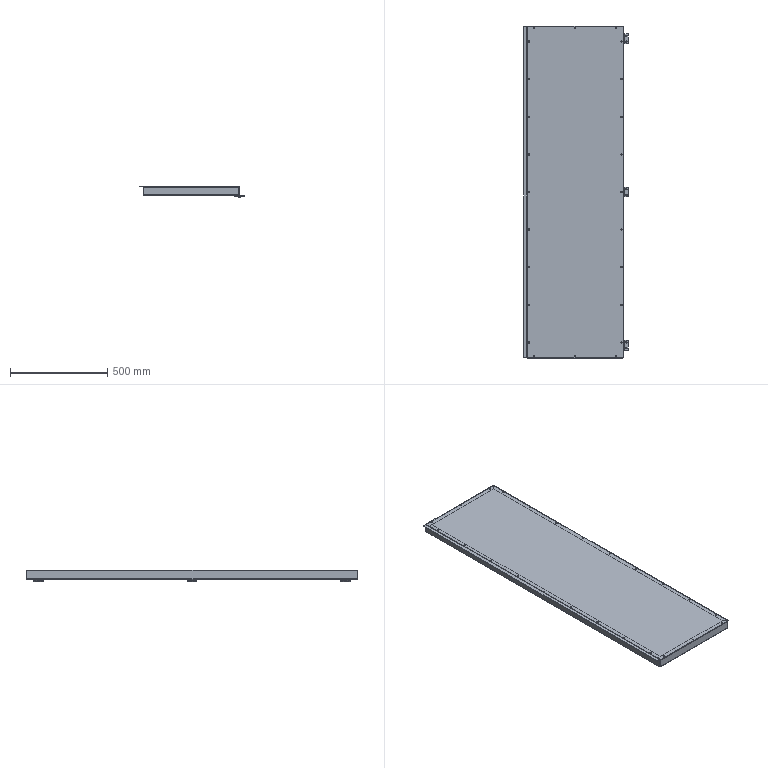Part | SolidWorks | 9 solids | 406 faces | box 537 x 1703 x 59.5 mm | volume 4565444 mm3 | cylinder 196 | plane 174 | cone 24 | spline 12 | commonest cylinder face diameters 5 x60 6.5 x48 6 x24 6.3 x24 12 x24 1.473 x8